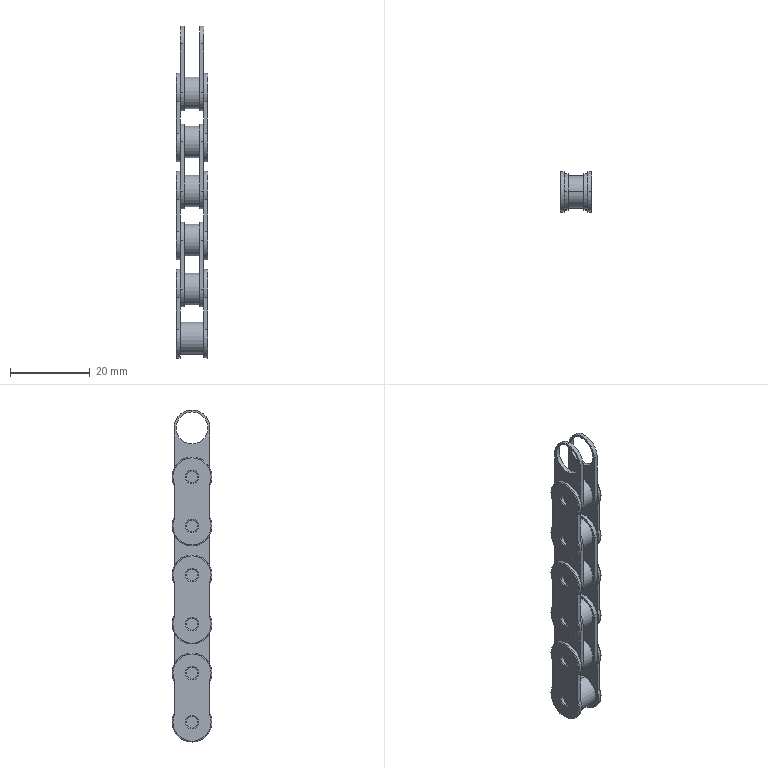Part | STEP file | 3 Chain Links v2 | 3 solids | 198 faces | box 8 x 10 x 83.3 mm | volume 3317 mm3 | cylinder 96 | plane 60 | torus 42 | commonest cylinder face diameters 3 x24 8 x24 9 x18 10 x18 0.4 x12